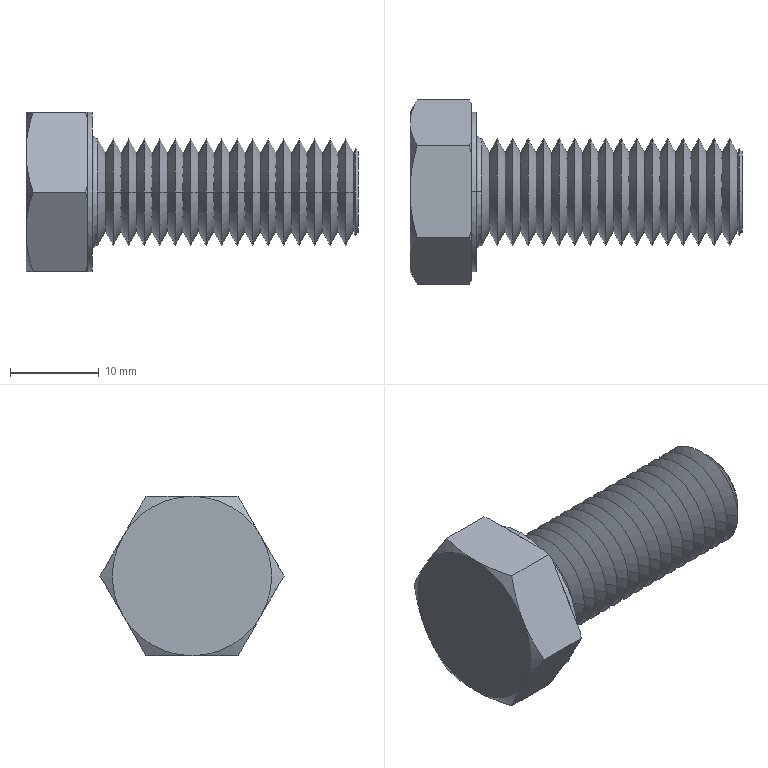Part | SolidWorks | features RevCut 4, Chamfer 1, Extrusion 1, Fillet 1, LPattern 1, Revolution 1 | 1 solid | 133 faces | box 37.5 x 20.785 x 18 mm | volume 4700 mm3 | cone 82 | cylinder 34 | plane 15 | torus 2 | commonest cylinder face diameters 12 x32 18 x2